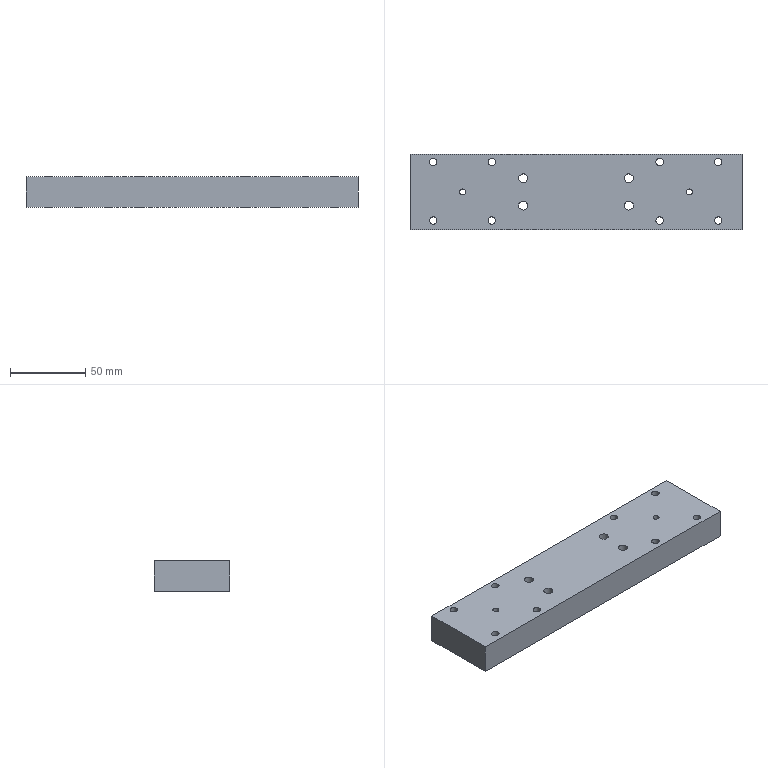Part | NX | 1 solid | 20 faces | box 220 x 50 x 20 mm | volume 214094 mm3 | cylinder 14 | plane 6 | commonest cylinder face diameters 5 x8 6 x4 4 x2
STEP:
#1=CARTESIAN_POINT('',(110.,25.,-20.));
#2=VERTEX_POINT('',#1);
#3=CARTESIAN_POINT('',(-110.,25.,-20.));
#4=VERTEX_POINT('',#3);
#5=CARTESIAN_POINT('',(110.,25.,-20.));
#6=DIRECTION('',(-1.,0.,0.));
#7=VECTOR('',#6,1000.);
#8=LINE('',#5,#7);
#9=EDGE_CURVE('',#2,#4,#8,.T.);
#10=ORIENTED_EDGE('',*,*,#9,.T.);
#11=CARTESIAN_POINT('',(-110.,25.,0.));
#12=VERTEX_POINT('',#11);
#13=CARTESIAN_POINT('',(-110.,25.,0.));
#14=DIRECTION('',(0.,0.,-1.));
#15=VECTOR('',#14,1000.);
#16=LINE('',#13,#15);
#17=EDGE_CURVE('',#4,#12,#16,.F.);
#18=ORIENTED_EDGE('',*,*,#17,.T.);
#19=CARTESIAN_POINT('',(110.,25.,0.));
#20=VERTEX_POINT('',#19);
#21=CARTESIAN_POINT('',(110.,25.,0.));
#22=DIRECTION('',(-1.,0.,0.));
#23=VECTOR('',#22,1000.);
#24=LINE('',#21,#23);
#25=EDGE_CURVE('',#12,#20,#24,.F.);
#26=ORIENTED_EDGE('',*,*,#25,.T.);
#27=CARTESIAN_POINT('',(110.,25.,0.));
#28=DIRECTION('',(0.,0.,-1.));
#29=VECTOR('',#28,1000.);
#30=LINE('',#27,#29);
#31=EDGE_CURVE('',#20,#2,#30,.T.);
#32=ORIENTED_EDGE('',*,*,#31,.T.);
#33=EDGE_LOOP('',(#10,#18,#26,#32));
#34=FACE_BOUND('',#33,.T.);
#35=CARTESIAN_POINT('',(110.,25.,0.));
#36=DIRECTION('',(0.,-1.,0.));
#37=DIRECTION('',(1.,0.,0.));
#38=AXIS2_PLACEMENT_3D('',#35,#36,#37);
#39=PLANE('',#38);
#40=ADVANCED_FACE('',(#34),#39,.F.);
#41=CARTESIAN_POINT('',(-110.,-25.,-20.));
#42=VERTEX_POINT('',#41);
#43=CARTESIAN_POINT('',(-110.,25.,-20.));
#44=DIRECTION('',(0.,-1.,0.));
#45=VECTOR('',#44,1000.);
#46=LINE('',#43,#45);
#47=EDGE_CURVE('',#4,#42,#46,.T.);
#48=ORIENTED_EDGE('',*,*,#47,.T.);
#49=CARTESIAN_POINT('',(-110.,-25.,0.));
#50=VERTEX_POINT('',#49);
#51=CARTESIAN_POINT('',(-110.,-25.,0.));
#52=DIRECTION('',(0.,0.,-1.));
#53=VECTOR('',#52,1000.);
#54=LINE('',#51,#53);
#55=EDGE_CURVE('',#50,#42,#54,.T.);
#56=ORIENTED_EDGE('',*,*,#55,.F.);
#57=CARTESIAN_POINT('',(-110.,25.,0.));
#58=DIRECTION('',(0.,-1.,0.));
#59=VECTOR('',#58,1000.);
#60=LINE('',#57,#59);
#61=EDGE_CURVE('',#12,#50,#60,.T.);
#62=ORIENTED_EDGE('',*,*,#61,.F.);
#63=ORIENTED_EDGE('',*,*,#17,.F.);
#64=EDGE_LOOP('',(#48,#56,#62,#63));
#65=FACE_BOUND('',#64,.T.);
#66=CARTESIAN_POINT('',(-110.,25.,0.));
#67=DIRECTION('',(1.,0.,0.));
#68=DIRECTION('',(0.,0.,1.));
#69=AXIS2_PLACEMENT_3D('',#66,#67,#68);
#70=PLANE('',#69);
#71=ADVANCED_FACE('',(#65),#70,.F.);
#72=CARTESIAN_POINT('',(110.,-25.,-20.));
#73=VERTEX_POINT('',#72);
#74=CARTESIAN_POINT('',(110.,-25.,-20.));
#75=DIRECTION('',(1.,0.,0.));
#76=VECTOR('',#75,1000.);
#77=LINE('',#74,#76);
#78=EDGE_CURVE('',#42,#73,#77,.T.);
#79=ORIENTED_EDGE('',*,*,#78,.T.);
#80=CARTESIAN_POINT('',(110.,-25.,0.));
#81=VERTEX_POINT('',#80);
#82=CARTESIAN_POINT('',(110.,-25.,0.));
#83=DIRECTION('',(0.,0.,-1.));
#84=VECTOR('',#83,1000.);
#85=LINE('',#82,#84);
#86=EDGE_CURVE('',#81,#73,#85,.T.);
#87=ORIENTED_EDGE('',*,*,#86,.F.);
#88=CARTESIAN_POINT('',(110.,-25.,0.));
#89=DIRECTION('',(1.,0.,0.));
#90=VECTOR('',#89,1000.);
#91=LINE('',#88,#90);
#92=EDGE_CURVE('',#50,#81,#91,.T.);
#93=ORIENTED_EDGE('',*,*,#92,.F.);
#94=ORIENTED_EDGE('',*,*,#55,.T.);
#95=EDGE_LOOP('',(#79,#87,#93,#94));
#96=FACE_BOUND('',#95,.T.);
#97=CARTESIAN_POINT('',(110.,-25.,0.));
#98=DIRECTION('',(0.,1.,0.));
#99=DIRECTION('',(-1.,0.,0.));
#100=AXIS2_PLACEMENT_3D('',#97,#98,#99);
#101=PLANE('',#100);
#102=ADVANCED_FACE('',(#96),#101,.F.);
#103=CARTESIAN_POINT('',(110.,25.,-20.));
#104=DIRECTION('',(0.,1.,0.));
#105=VECTOR('',#104,1000.);
#106=LINE('',#103,#105);
#107=EDGE_CURVE('',#73,#2,#106,.T.);
#108=ORIENTED_EDGE('',*,*,#107,.T.);
#109=ORIENTED_EDGE('',*,*,#31,.F.);
#110=CARTESIAN_POINT('',(110.,25.,0.));
#111=DIRECTION('',(0.,1.,0.));
#112=VECTOR('',#111,1000.);
#113=LINE('',#110,#112);
#114=EDGE_CURVE('',#81,#20,#113,.T.);
#115=ORIENTED_EDGE('',*,*,#114,.F.);
#116=ORIENTED_EDGE('',*,*,#86,.T.);
#117=EDGE_LOOP('',(#108,#109,#115,#116));
#118=FACE_BOUND('',#117,.T.);
#119=CARTESIAN_POINT('',(110.,25.,0.));
#120=DIRECTION('',(-1.,0.,0.));
#121=DIRECTION('',(0.,0.,-1.));
#122=AXIS2_PLACEMENT_3D('',#119,#120,#121);
#123=PLANE('',#122);
#124=ADVANCED_FACE('',(#118),#123,.F.);
#125=CARTESIAN_POINT('',(94.255,-16.487,0.));
#126=VERTEX_POINT('',#125);
#127=CARTESIAN_POINT('',(94.255,-18.987,0.));
#128=DIRECTION('',(0.,0.,-1.));
#129=DIRECTION('',(0.,1.,0.));
#130=AXIS2_PLACEMENT_3D('',#127,#128,#129);
#131=CIRCLE('',#130,2.5);
#132=EDGE_CURVE('',#126,#126,#131,.T.);
#133=ORIENTED_EDGE('',*,*,#132,.T.);
#134=EDGE_LOOP('',(#133));
#135=FACE_BOUND('',#134,.T.);
#136=CARTESIAN_POINT('',(94.255,22.404,0.));
#137=VERTEX_POINT('',#136);
#138=CARTESIAN_POINT('',(94.255,19.904,0.));
#139=DIRECTION('',(0.,0.,-1.));
#140=DIRECTION('',(0.,1.,0.));
#141=AXIS2_PLACEMENT_3D('',#138,#139,#140);
#142=CIRCLE('',#141,2.5);
#143=EDGE_CURVE('',#137,#137,#142,.T.);
#144=ORIENTED_EDGE('',*,*,#143,.T.);
#145=EDGE_LOOP('',(#144));
#146=FACE_BOUND('',#145,.T.);
#147=CARTESIAN_POINT('',(55.365,-16.487,0.));
#148=VERTEX_POINT('',#147);
#149=CARTESIAN_POINT('',(55.365,-18.987,0.));
#150=DIRECTION('',(0.,0.,-1.));
#151=DIRECTION('',(0.,1.,0.));
#152=AXIS2_PLACEMENT_3D('',#149,#150,#151);
#153=CIRCLE('',#152,2.5);
#154=EDGE_CURVE('',#148,#148,#153,.T.);
#155=ORIENTED_EDGE('',*,*,#154,.T.);
#156=EDGE_LOOP('',(#155));
#157=FACE_BOUND('',#156,.T.);
#158=CARTESIAN_POINT('',(55.365,22.404,0.));
#159=VERTEX_POINT('',#158);
#160=CARTESIAN_POINT('',(55.365,19.904,0.));
#161=DIRECTION('',(0.,0.,-1.));
#162=DIRECTION('',(0.,1.,0.));
#163=AXIS2_PLACEMENT_3D('',#160,#161,#162);
#164=CIRCLE('',#163,2.5);
#165=EDGE_CURVE('',#159,#159,#164,.T.);
#166=ORIENTED_EDGE('',*,*,#165,.T.);
#167=EDGE_LOOP('',(#166));
#168=FACE_BOUND('',#167,.T.);
#169=CARTESIAN_POINT('',(-55.745,-16.487,0.));
#170=VERTEX_POINT('',#169);
#171=CARTESIAN_POINT('',(-55.745,-18.987,0.));
#172=DIRECTION('',(0.,0.,-1.));
#173=DIRECTION('',(0.,1.,0.));
#174=AXIS2_PLACEMENT_3D('',#171,#172,#173);
#175=CIRCLE('',#174,2.5);
#176=EDGE_CURVE('',#170,#170,#175,.T.);
#177=ORIENTED_EDGE('',*,*,#176,.T.);
#178=EDGE_LOOP('',(#177));
#179=FACE_BOUND('',#178,.T.);
#180=CARTESIAN_POINT('',(-55.745,22.404,0.));
#181=VERTEX_POINT('',#180);
#182=CARTESIAN_POINT('',(-55.745,19.904,0.));
#183=DIRECTION('',(0.,0.,-1.));
#184=DIRECTION('',(0.,1.,0.));
#185=AXIS2_PLACEMENT_3D('',#182,#183,#184);
#186=CIRCLE('',#185,2.5);
#187=EDGE_CURVE('',#181,#181,#186,.T.);
#188=ORIENTED_EDGE('',*,*,#187,.T.);
#189=EDGE_LOOP('',(#188));
#190=FACE_BOUND('',#189,.T.);
#191=CARTESIAN_POINT('',(-94.635,-16.487,0.));
#192=VERTEX_POINT('',#191);
#193=CARTESIAN_POINT('',(-94.635,-18.987,0.));
#194=DIRECTION('',(0.,0.,-1.));
#195=DIRECTION('',(0.,1.,0.));
#196=AXIS2_PLACEMENT_3D('',#193,#194,#195);
#197=CIRCLE('',#196,2.5);
#198=EDGE_CURVE('',#192,#192,#197,.T.);
#199=ORIENTED_EDGE('',*,*,#198,.T.);
#200=EDGE_LOOP('',(#199));
#201=FACE_BOUND('',#200,.T.);
#202=CARTESIAN_POINT('',(-94.635,22.404,0.));
#203=VERTEX_POINT('',#202);
#204=CARTESIAN_POINT('',(-94.635,19.904,0.));
#205=DIRECTION('',(0.,0.,-1.));
#206=DIRECTION('',(0.,1.,0.));
#207=AXIS2_PLACEMENT_3D('',#204,#205,#206);
#208=CIRCLE('',#207,2.5);
#209=EDGE_CURVE('',#203,#203,#208,.T.);
#210=ORIENTED_EDGE('',*,*,#209,.T.);
#211=EDGE_LOOP('',(#210));
#212=FACE_BOUND('',#211,.T.);
#213=CARTESIAN_POINT('',(-75.,2.,0.));
#214=VERTEX_POINT('',#213);
#215=CARTESIAN_POINT('',(-75.,0.,0.));
#216=DIRECTION('',(0.,0.,-1.));
#217=DIRECTION('',(0.,1.,0.));
#218=AXIS2_PLACEMENT_3D('',#215,#216,#217);
#219=CIRCLE('',#218,2.);
#220=EDGE_CURVE('',#214,#214,#219,.T.);
#221=ORIENTED_EDGE('',*,*,#220,.T.);
#222=EDGE_LOOP('',(#221));
#223=FACE_BOUND('',#222,.T.);
#224=CARTESIAN_POINT('',(75.,2.,0.));
#225=VERTEX_POINT('',#224);
#226=CARTESIAN_POINT('',(75.,0.,0.));
#227=DIRECTION('',(0.,0.,-1.));
#228=DIRECTION('',(0.,1.,0.));
#229=AXIS2_PLACEMENT_3D('',#226,#227,#228);
#230=CIRCLE('',#229,2.);
#231=EDGE_CURVE('',#225,#225,#230,.T.);
#232=ORIENTED_EDGE('',*,*,#231,.T.);
#233=EDGE_LOOP('',(#232));
#234=FACE_BOUND('',#233,.T.);
#235=CARTESIAN_POINT('',(35.,-12.,0.));
#236=VERTEX_POINT('',#235);
#237=CARTESIAN_POINT('',(35.,-9.,0.));
#238=DIRECTION('',(0.,0.,1.));
#239=DIRECTION('',(0.,-1.,0.));
#240=AXIS2_PLACEMENT_3D('',#237,#238,#239);
#241=CIRCLE('',#240,3.);
#242=EDGE_CURVE('',#236,#236,#241,.T.);
#243=ORIENTED_EDGE('',*,*,#242,.F.);
#244=EDGE_LOOP('',(#243));
#245=FACE_BOUND('',#244,.T.);
#246=CARTESIAN_POINT('',(-35.,6.,0.));
#247=VERTEX_POINT('',#246);
#248=CARTESIAN_POINT('',(-35.,9.,0.));
#249=DIRECTION('',(0.,0.,1.));
#250=DIRECTION('',(0.,-1.,0.));
#251=AXIS2_PLACEMENT_3D('',#248,#249,#250);
#252=CIRCLE('',#251,3.);
#253=EDGE_CURVE('',#247,#247,#252,.T.);
#254=ORIENTED_EDGE('',*,*,#253,.F.);
#255=EDGE_LOOP('',(#254));
#256=FACE_BOUND('',#255,.T.);
#257=CARTESIAN_POINT('',(-35.,-12.,0.));
#258=VERTEX_POINT('',#257);
#259=CARTESIAN_POINT('',(-35.,-9.,0.));
#260=DIRECTION('',(0.,0.,1.));
#261=DIRECTION('',(0.,-1.,0.));
#262=AXIS2_PLACEMENT_3D('',#259,#260,#261);
#263=CIRCLE('',#262,3.);
#264=EDGE_CURVE('',#258,#258,#263,.T.);
#265=ORIENTED_EDGE('',*,*,#264,.F.);
#266=EDGE_LOOP('',(#265));
#267=FACE_BOUND('',#266,.T.);
#268=CARTESIAN_POINT('',(35.,6.,0.));
#269=VERTEX_POINT('',#268);
#270=CARTESIAN_POINT('',(35.,9.,0.));
#271=DIRECTION('',(0.,0.,1.));
#272=DIRECTION('',(0.,-1.,0.));
#273=AXIS2_PLACEMENT_3D('',#270,#271,#272);
#274=CIRCLE('',#273,3.);
#275=EDGE_CURVE('',#269,#269,#274,.T.);
#276=ORIENTED_EDGE('',*,*,#275,.F.);
#277=EDGE_LOOP('',(#276));
#278=FACE_BOUND('',#277,.T.);
#279=ORIENTED_EDGE('',*,*,#25,.F.);
#280=ORIENTED_EDGE('',*,*,#61,.T.);
#281=ORIENTED_EDGE('',*,*,#92,.T.);
#282=ORIENTED_EDGE('',*,*,#114,.T.);
#283=EDGE_LOOP('',(#279,#280,#281,#282));
#284=FACE_BOUND('',#283,.T.);
#285=CARTESIAN_POINT('',(-300.39,133.654,0.));
#286=DIRECTION('',(0.,0.,1.));
#287=DIRECTION('',(0.,-1.,0.));
#288=AXIS2_PLACEMENT_3D('',#285,#286,#287);
#289=PLANE('',#288);
#290=ADVANCED_FACE('',(#135,#146,#157,#168,#179,#190,#201,#212,#223,#234,#245,#256,#267,#278,#284),#289,.T.);
#291=CARTESIAN_POINT('',(94.255,-16.487,-20.));
#292=VERTEX_POINT('',#291);
#293=CARTESIAN_POINT('',(94.255,-18.987,-20.));
#294=DIRECTION('',(0.,0.,-1.));
#295=DIRECTION('',(0.,1.,0.));
#296=AXIS2_PLACEMENT_3D('',#293,#294,#295);
#297=CIRCLE('',#296,2.5);
#298=EDGE_CURVE('',#292,#292,#297,.T.);
#299=ORIENTED_EDGE('',*,*,#298,.F.);
#300=EDGE_LOOP('',(#299));
#301=FACE_BOUND('',#300,.T.);
#302=CARTESIAN_POINT('',(94.255,22.404,-20.));
#303=VERTEX_POINT('',#302);
#304=CARTESIAN_POINT('',(94.255,19.904,-20.));
#305=DIRECTION('',(0.,0.,-1.));
#306=DIRECTION('',(0.,1.,0.));
#307=AXIS2_PLACEMENT_3D('',#304,#305,#306);
#308=CIRCLE('',#307,2.5);
#309=EDGE_CURVE('',#303,#303,#308,.T.);
#310=ORIENTED_EDGE('',*,*,#309,.F.);
#311=EDGE_LOOP('',(#310));
#312=FACE_BOUND('',#311,.T.);
#313=CARTESIAN_POINT('',(55.365,-16.487,-20.));
#314=VERTEX_POINT('',#313);
#315=CARTESIAN_POINT('',(55.365,-18.987,-20.));
#316=DIRECTION('',(0.,0.,-1.));
#317=DIRECTION('',(0.,1.,0.));
#318=AXIS2_PLACEMENT_3D('',#315,#316,#317);
#319=CIRCLE('',#318,2.5);
#320=EDGE_CURVE('',#314,#314,#319,.T.);
#321=ORIENTED_EDGE('',*,*,#320,.F.);
#322=EDGE_LOOP('',(#321));
#323=FACE_BOUND('',#322,.T.);
#324=CARTESIAN_POINT('',(55.365,22.404,-20.));
#325=VERTEX_POINT('',#324);
#326=CARTESIAN_POINT('',(55.365,19.904,-20.));
#327=DIRECTION('',(0.,0.,-1.));
#328=DIRECTION('',(0.,1.,0.));
#329=AXIS2_PLACEMENT_3D('',#326,#327,#328);
#330=CIRCLE('',#329,2.5);
#331=EDGE_CURVE('',#325,#325,#330,.T.);
#332=ORIENTED_EDGE('',*,*,#331,.F.);
#333=EDGE_LOOP('',(#332));
#334=FACE_BOUND('',#333,.T.);
#335=CARTESIAN_POINT('',(-55.745,-16.487,-20.));
#336=VERTEX_POINT('',#335);
#337=CARTESIAN_POINT('',(-55.745,-18.987,-20.));
#338=DIRECTION('',(0.,0.,-1.));
#339=DIRECTION('',(0.,1.,0.));
#340=AXIS2_PLACEMENT_3D('',#337,#338,#339);
#341=CIRCLE('',#340,2.5);
#342=EDGE_CURVE('',#336,#336,#341,.T.);
#343=ORIENTED_EDGE('',*,*,#342,.F.);
#344=EDGE_LOOP('',(#343));
#345=FACE_BOUND('',#344,.T.);
#346=CARTESIAN_POINT('',(-55.745,22.404,-20.));
#347=VERTEX_POINT('',#346);
#348=CARTESIAN_POINT('',(-55.745,19.904,-20.));
#349=DIRECTION('',(0.,0.,-1.));
#350=DIRECTION('',(0.,1.,0.));
#351=AXIS2_PLACEMENT_3D('',#348,#349,#350);
#352=CIRCLE('',#351,2.5);
#353=EDGE_CURVE('',#347,#347,#352,.T.);
#354=ORIENTED_EDGE('',*,*,#353,.F.);
#355=EDGE_LOOP('',(#354));
#356=FACE_BOUND('',#355,.T.);
#357=CARTESIAN_POINT('',(-94.635,-16.487,-20.));
#358=VERTEX_POINT('',#357);
#359=CARTESIAN_POINT('',(-94.635,-18.987,-20.));
#360=DIRECTION('',(0.,0.,-1.));
#361=DIRECTION('',(0.,1.,0.));
#362=AXIS2_PLACEMENT_3D('',#359,#360,#361);
#363=CIRCLE('',#362,2.5);
#364=EDGE_CURVE('',#358,#358,#363,.T.);
#365=ORIENTED_EDGE('',*,*,#364,.F.);
#366=EDGE_LOOP('',(#365));
#367=FACE_BOUND('',#366,.T.);
#368=CARTESIAN_POINT('',(-94.635,22.404,-20.));
#369=VERTEX_POINT('',#368);
#370=CARTESIAN_POINT('',(-94.635,19.904,-20.));
#371=DIRECTION('',(0.,0.,-1.));
#372=DIRECTION('',(0.,1.,0.));
#373=AXIS2_PLACEMENT_3D('',#370,#371,#372);
#374=CIRCLE('',#373,2.5);
#375=EDGE_CURVE('',#369,#369,#374,.T.);
#376=ORIENTED_EDGE('',*,*,#375,.F.);
#377=EDGE_LOOP('',(#376));
#378=FACE_BOUND('',#377,.T.);
#379=CARTESIAN_POINT('',(-75.,2.,-20.));
#380=VERTEX_POINT('',#379);
#381=CARTESIAN_POINT('',(-75.,0.,-20.));
#382=DIRECTION('',(0.,0.,-1.));
#383=DIRECTION('',(0.,1.,0.));
#384=AXIS2_PLACEMENT_3D('',#381,#382,#383);
#385=CIRCLE('',#384,2.);
#386=EDGE_CURVE('',#380,#380,#385,.T.);
#387=ORIENTED_EDGE('',*,*,#386,.F.);
#388=EDGE_LOOP('',(#387));
#389=FACE_BOUND('',#388,.T.);
#390=CARTESIAN_POINT('',(75.,2.,-20.));
#391=VERTEX_POINT('',#390);
#392=CARTESIAN_POINT('',(75.,0.,-20.));
#393=DIRECTION('',(0.,0.,-1.));
#394=DIRECTION('',(0.,1.,0.));
#395=AXIS2_PLACEMENT_3D('',#392,#393,#394);
#396=CIRCLE('',#395,2.);
#397=EDGE_CURVE('',#391,#391,#396,.T.);
#398=ORIENTED_EDGE('',*,*,#397,.F.);
#399=EDGE_LOOP('',(#398));
#400=FACE_BOUND('',#399,.T.);
#401=CARTESIAN_POINT('',(35.,-12.,-20.));
#402=VERTEX_POINT('',#401);
#403=CARTESIAN_POINT('',(35.,-9.,-20.));
#404=DIRECTION('',(0.,0.,1.));
#405=DIRECTION('',(0.,-1.,0.));
#406=AXIS2_PLACEMENT_3D('',#403,#404,#405);
#407=CIRCLE('',#406,3.);
#408=EDGE_CURVE('',#402,#402,#407,.T.);
#409=ORIENTED_EDGE('',*,*,#408,.T.);
#410=EDGE_LOOP('',(#409));
#411=FACE_BOUND('',#410,.T.);
#412=CARTESIAN_POINT('',(-35.,6.,-20.));
#413=VERTEX_POINT('',#412);
#414=CARTESIAN_POINT('',(-35.,9.,-20.));
#415=DIRECTION('',(0.,0.,1.));
#416=DIRECTION('',(0.,-1.,0.));
#417=AXIS2_PLACEMENT_3D('',#414,#415,#416);
#418=CIRCLE('',#417,3.);
#419=EDGE_CURVE('',#413,#413,#418,.T.);
#420=ORIENTED_EDGE('',*,*,#419,.T.);
#421=EDGE_LOOP('',(#420));
#422=FACE_BOUND('',#421,.T.);
#423=CARTESIAN_POINT('',(-35.,-12.,-20.));
#424=VERTEX_POINT('',#423);
#425=CARTESIAN_POINT('',(-35.,-9.,-20.));
#426=DIRECTION('',(0.,0.,1.));
#427=DIRECTION('',(0.,-1.,0.));
#428=AXIS2_PLACEMENT_3D('',#425,#426,#427);
#429=CIRCLE('',#428,3.);
#430=EDGE_CURVE('',#424,#424,#429,.T.);
#431=ORIENTED_EDGE('',*,*,#430,.T.);
#432=EDGE_LOOP('',(#431));
#433=FACE_BOUND('',#432,.T.);
#434=CARTESIAN_POINT('',(35.,6.,-20.));
#435=VERTEX_POINT('',#434);
#436=CARTESIAN_POINT('',(35.,9.,-20.));
#437=DIRECTION('',(0.,0.,1.));
#438=DIRECTION('',(0.,-1.,0.));
#439=AXIS2_PLACEMENT_3D('',#436,#437,#438);
#440=CIRCLE('',#439,3.);
#441=EDGE_CURVE('',#435,#435,#440,.T.);
#442=ORIENTED_EDGE('',*,*,#441,.T.);
#443=EDGE_LOOP('',(#442));
#444=FACE_BOUND('',#443,.T.);
#445=ORIENTED_EDGE('',*,*,#9,.F.);
#446=ORIENTED_EDGE('',*,*,#107,.F.);
#447=ORIENTED_EDGE('',*,*,#78,.F.);
#448=ORIENTED_EDGE('',*,*,#47,.F.);
#449=EDGE_LOOP('',(#445,#446,#447,#448));
#450=FACE_BOUND('',#449,.T.);
#451=CARTESIAN_POINT('',(-300.39,133.654,-20.));
#452=DIRECTION('',(0.,0.,1.));
#453=DIRECTION('',(0.,-1.,0.));
#454=AXIS2_PLACEMENT_3D('',#451,#452,#453);
#455=PLANE('',#454);
#456=ADVANCED_FACE('',(#301,#312,#323,#334,#345,#356,#367,#378,#389,#400,#411,#422,#433,#444,#450),#455,.F.);
#457=ORIENTED_EDGE('',*,*,#441,.F.);
#458=EDGE_LOOP('',(#457));
#459=FACE_BOUND('',#458,.T.);
#460=ORIENTED_EDGE('',*,*,#275,.T.);
#461=EDGE_LOOP('',(#460));
#462=FACE_BOUND('',#461,.T.);
#463=CARTESIAN_POINT('',(35.,9.,-20.));
#464=DIRECTION('',(0.,0.,1.));
#465=DIRECTION('',(0.,-1.,0.));
#466=AXIS2_PLACEMENT_3D('',#463,#464,#465);
#467=CYLINDRICAL_SURFACE('',#466,3.);
#468=ADVANCED_FACE('',(#459,#462),#467,.F.);
#469=ORIENTED_EDGE('',*,*,#430,.F.);
#470=EDGE_LOOP('',(#469));
#471=FACE_BOUND('',#470,.T.);
#472=ORIENTED_EDGE('',*,*,#264,.T.);
#473=EDGE_LOOP('',(#472));
#474=FACE_BOUND('',#473,.T.);
#475=CARTESIAN_POINT('',(-35.,-9.,-20.));
#476=DIRECTION('',(0.,0.,1.));
#477=DIRECTION('',(0.,-1.,0.));
#478=AXIS2_PLACEMENT_3D('',#475,#476,#477);
#479=CYLINDRICAL_SURFACE('',#478,3.);
#480=ADVANCED_FACE('',(#471,#474),#479,.F.);
#481=ORIENTED_EDGE('',*,*,#419,.F.);
#482=EDGE_LOOP('',(#481));
#483=FACE_BOUND('',#482,.T.);
#484=ORIENTED_EDGE('',*,*,#253,.T.);
#485=EDGE_LOOP('',(#484));
#486=FACE_BOUND('',#485,.T.);
#487=CARTESIAN_POINT('',(-35.,9.,-20.));
#488=DIRECTION('',(0.,0.,1.));
#489=DIRECTION('',(0.,-1.,0.));
#490=AXIS2_PLACEMENT_3D('',#487,#488,#489);
#491=CYLINDRICAL_SURFACE('',#490,3.);
#492=ADVANCED_FACE('',(#483,#486),#491,.F.);
#493=ORIENTED_EDGE('',*,*,#408,.F.);
#494=EDGE_LOOP('',(#493));
#495=FACE_BOUND('',#494,.T.);
#496=ORIENTED_EDGE('',*,*,#242,.T.);
#497=EDGE_LOOP('',(#496));
#498=FACE_BOUND('',#497,.T.);
#499=CARTESIAN_POINT('',(35.,-9.,-20.));
#500=DIRECTION('',(0.,0.,1.));
#501=DIRECTION('',(0.,-1.,0.));
#502=AXIS2_PLACEMENT_3D('',#499,#500,#501);
#503=CYLINDRICAL_SURFACE('',#502,3.);
#504=ADVANCED_FACE('',(#495,#498),#503,.F.);
#505=ORIENTED_EDGE('',*,*,#231,.F.);
#506=EDGE_LOOP('',(#505));
#507=FACE_BOUND('',#506,.T.);
#508=ORIENTED_EDGE('',*,*,#397,.T.);
#509=EDGE_LOOP('',(#508));
#510=FACE_BOUND('',#509,.T.);
#511=CARTESIAN_POINT('',(75.,0.,0.));
#512=DIRECTION('',(0.,0.,-1.));
#513=DIRECTION('',(0.,1.,0.));
#514=AXIS2_PLACEMENT_3D('',#511,#512,#513);
#515=CYLINDRICAL_SURFACE('',#514,2.);
#516=ADVANCED_FACE('',(#507,#510),#515,.F.);
#517=ORIENTED_EDGE('',*,*,#220,.F.);
#518=EDGE_LOOP('',(#517));
#519=FACE_BOUND('',#518,.T.);
#520=ORIENTED_EDGE('',*,*,#386,.T.);
#521=EDGE_LOOP('',(#520));
#522=FACE_BOUND('',#521,.T.);
#523=CARTESIAN_POINT('',(-75.,0.,0.));
#524=DIRECTION('',(0.,0.,-1.));
#525=DIRECTION('',(0.,1.,0.));
#526=AXIS2_PLACEMENT_3D('',#523,#524,#525);
#527=CYLINDRICAL_SURFACE('',#526,2.);
#528=ADVANCED_FACE('',(#519,#522),#527,.F.);
#529=ORIENTED_EDGE('',*,*,#209,.F.);
#530=EDGE_LOOP('',(#529));
#531=FACE_BOUND('',#530,.T.);
#532=ORIENTED_EDGE('',*,*,#375,.T.);
#533=EDGE_LOOP('',(#532));
#534=FACE_BOUND('',#533,.T.);
#535=CARTESIAN_POINT('',(-94.635,19.904,0.));
#536=DIRECTION('',(0.,0.,-1.));
#537=DIRECTION('',(0.,1.,0.));
#538=AXIS2_PLACEMENT_3D('',#535,#536,#537);
#539=CYLINDRICAL_SURFACE('',#538,2.5);
#540=ADVANCED_FACE('',(#531,#534),#539,.F.);
#541=ORIENTED_EDGE('',*,*,#198,.F.);
#542=EDGE_LOOP('',(#541));
#543=FACE_BOUND('',#542,.T.);
#544=ORIENTED_EDGE('',*,*,#364,.T.);
#545=EDGE_LOOP('',(#544));
#546=FACE_BOUND('',#545,.T.);
#547=CARTESIAN_POINT('',(-94.635,-18.987,0.));
#548=DIRECTION('',(0.,0.,-1.));
#549=DIRECTION('',(0.,1.,0.));
#550=AXIS2_PLACEMENT_3D('',#547,#548,#549);
#551=CYLINDRICAL_SURFACE('',#550,2.5);
#552=ADVANCED_FACE('',(#543,#546),#551,.F.);
#553=ORIENTED_EDGE('',*,*,#187,.F.);
#554=EDGE_LOOP('',(#553));
#555=FACE_BOUND('',#554,.T.);
#556=ORIENTED_EDGE('',*,*,#353,.T.);
#557=EDGE_LOOP('',(#556));
#558=FACE_BOUND('',#557,.T.);
#559=CARTESIAN_POINT('',(-55.745,19.904,0.));
#560=DIRECTION('',(0.,0.,-1.));
#561=DIRECTION('',(0.,1.,0.));
#562=AXIS2_PLACEMENT_3D('',#559,#560,#561);
#563=CYLINDRICAL_SURFACE('',#562,2.5);
#564=ADVANCED_FACE('',(#555,#558),#563,.F.);
#565=ORIENTED_EDGE('',*,*,#176,.F.);
#566=EDGE_LOOP('',(#565));
#567=FACE_BOUND('',#566,.T.);
#568=ORIENTED_EDGE('',*,*,#342,.T.);
#569=EDGE_LOOP('',(#568));
#570=FACE_BOUND('',#569,.T.);
#571=CARTESIAN_POINT('',(-55.745,-18.987,0.));
#572=DIRECTION('',(0.,0.,-1.));
#573=DIRECTION('',(0.,1.,0.));
#574=AXIS2_PLACEMENT_3D('',#571,#572,#573);
#575=CYLINDRICAL_SURFACE('',#574,2.5);
#576=ADVANCED_FACE('',(#567,#570),#575,.F.);
#577=ORIENTED_EDGE('',*,*,#165,.F.);
#578=EDGE_LOOP('',(#577));
#579=FACE_BOUND('',#578,.T.);
#580=ORIENTED_EDGE('',*,*,#331,.T.);
#581=EDGE_LOOP('',(#580));
#582=FACE_BOUND('',#581,.T.);
#583=CARTESIAN_POINT('',(55.365,19.904,0.));
#584=DIRECTION('',(0.,0.,-1.));
#585=DIRECTION('',(0.,1.,0.));
#586=AXIS2_PLACEMENT_3D('',#583,#584,#585);
#587=CYLINDRICAL_SURFACE('',#586,2.5);
#588=ADVANCED_FACE('',(#579,#582),#587,.F.);
#589=ORIENTED_EDGE('',*,*,#154,.F.);
#590=EDGE_LOOP('',(#589));
#591=FACE_BOUND('',#590,.T.);
#592=ORIENTED_EDGE('',*,*,#320,.T.);
#593=EDGE_LOOP('',(#592));
#594=FACE_BOUND('',#593,.T.);
#595=CARTESIAN_POINT('',(55.365,-18.987,0.));
#596=DIRECTION('',(0.,0.,-1.));
#597=DIRECTION('',(0.,1.,0.));
#598=AXIS2_PLACEMENT_3D('',#595,#596,#597);
#599=CYLINDRICAL_SURFACE('',#598,2.5);
#600=ADVANCED_FACE('',(#591,#594),#599,.F.);
#601=ORIENTED_EDGE('',*,*,#143,.F.);
#602=EDGE_LOOP('',(#601));
#603=FACE_BOUND('',#602,.T.);
#604=ORIENTED_EDGE('',*,*,#309,.T.);
#605=EDGE_LOOP('',(#604));
#606=FACE_BOUND('',#605,.T.);
#607=CARTESIAN_POINT('',(94.255,19.904,0.));
#608=DIRECTION('',(0.,0.,-1.));
#609=DIRECTION('',(0.,1.,0.));
#610=AXIS2_PLACEMENT_3D('',#607,#608,#609);
#611=CYLINDRICAL_SURFACE('',#610,2.5);
#612=ADVANCED_FACE('',(#603,#606),#611,.F.);
#613=ORIENTED_EDGE('',*,*,#132,.F.);
#614=EDGE_LOOP('',(#613));
#615=FACE_BOUND('',#614,.T.);
#616=ORIENTED_EDGE('',*,*,#298,.T.);
#617=EDGE_LOOP('',(#616));
#618=FACE_BOUND('',#617,.T.);
#619=CARTESIAN_POINT('',(94.255,-18.987,0.));
#620=DIRECTION('',(0.,0.,-1.));
#621=DIRECTION('',(0.,1.,0.));
#622=AXIS2_PLACEMENT_3D('',#619,#620,#621);
#623=CYLINDRICAL_SURFACE('',#622,2.5);
#624=ADVANCED_FACE('',(#615,#618),#623,.F.);
#625=CLOSED_SHELL('',(#40,#71,#102,#124,#290,#456,#468,#480,#492,#504,#516,#528,#540,#552,#564,#576,#588,#600,#612,#624));
#626=MANIFOLD_SOLID_BREP('',#625);
#627=(LENGTH_UNIT()NAMED_UNIT(*)SI_UNIT(.MILLI.,.METRE.));
#628=UNCERTAINTY_MEASURE_WITH_UNIT(LENGTH_MEASURE(0.00001),#627,'','');
#629=(NAMED_UNIT(*)PLANE_ANGLE_UNIT()SI_UNIT($,.RADIAN.));
#630=(NAMED_UNIT(*)SI_UNIT($,.STERADIAN.)SOLID_ANGLE_UNIT());
#631=(GEOMETRIC_REPRESENTATION_CONTEXT(3)GLOBAL_UNCERTAINTY_ASSIGNED_CONTEXT((#628))GLOBAL_UNIT_ASSIGNED_CONTEXT((#627,#629,#630))REPRESENTATION_CONTEXT('',''));
#632=ADVANCED_BREP_SHAPE_REPRESENTATION('',(#626),#631);